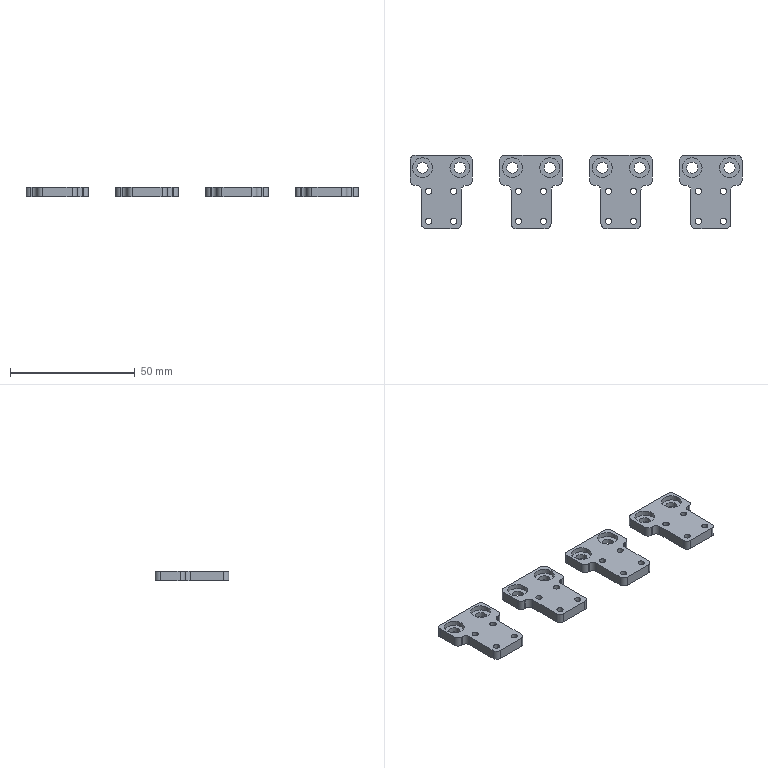Part | 4 solids | 112 faces | box 133 x 29.5 x 4 mm | volume 7852 mm3 | cylinder 64 | plane 48 | commonest cylinder face diameters 4 x32 2.5 x16 4.5 x8 8 x8